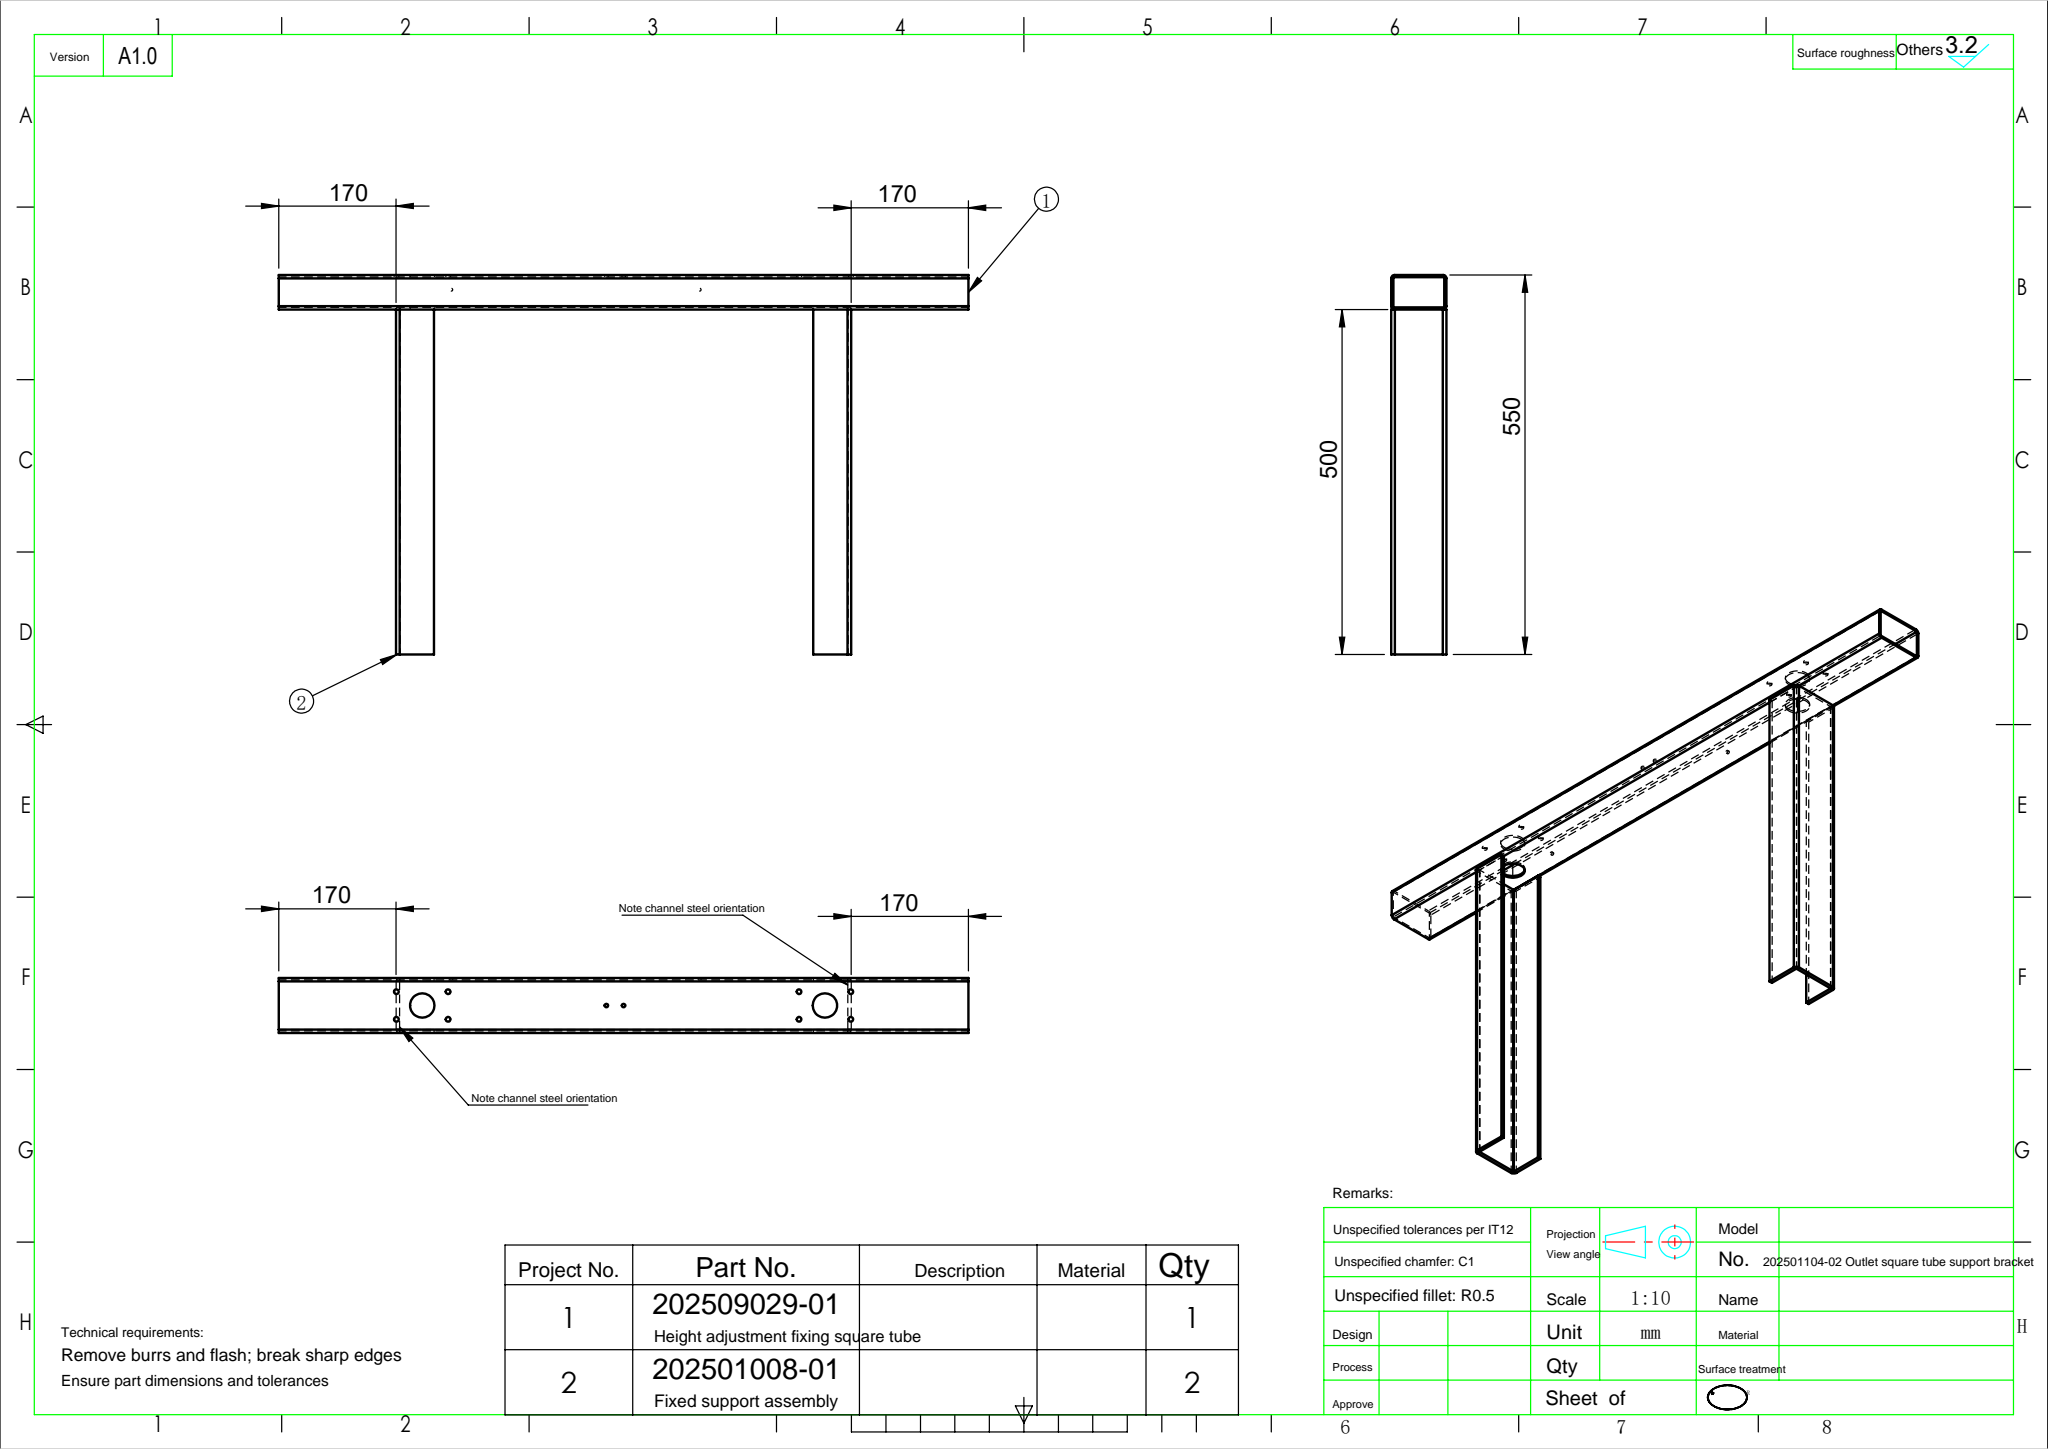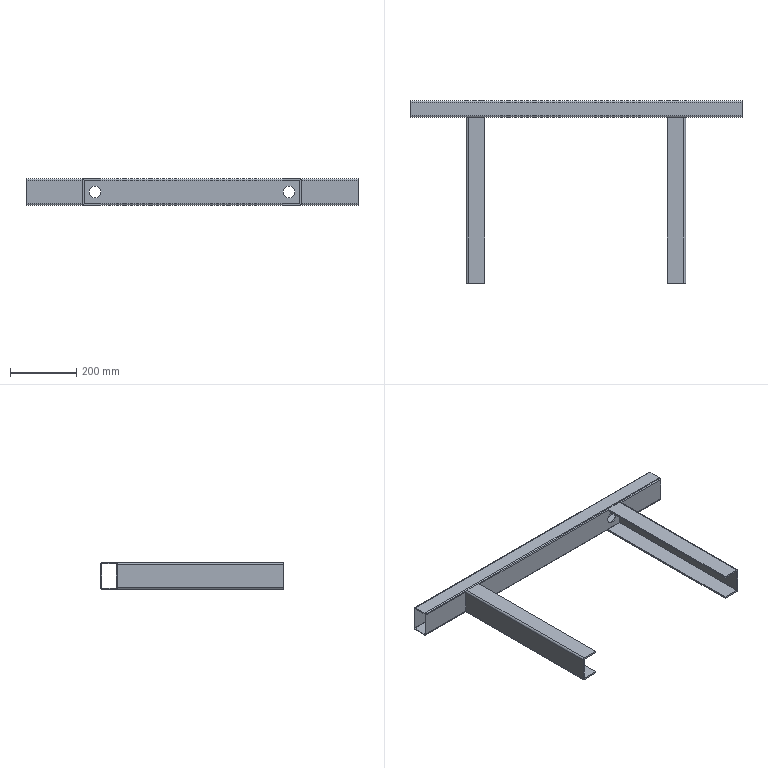Part | SolidWorks | 3 solids | 90 faces | box 1000 x 550 x 80 mm | volume 1598201 mm3 | plane 46 | cylinder 44 | commonest cylinder face diameters 6.8 x16 35.2 x8 0.4 x4 4.2 x4 5 x4 10 x4